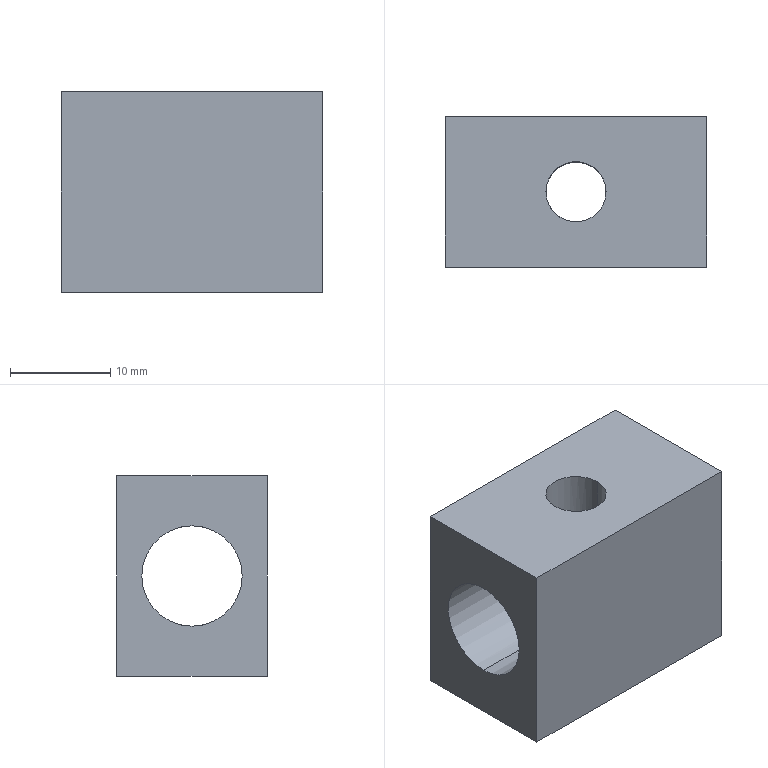Part | SolidWorks | features Extrusion 1, ICE 1 | 1 solid | 12 faces | box 26 x 15 x 20 mm | volume 5462 mm3 | cylinder 6 | plane 6 | commonest cylinder face diameters 6 x4 10 x2
STEP:
#1=CARTESIAN_POINT('',(-13.,0.,15.));
#2=VERTEX_POINT('',#1);
#3=CARTESIAN_POINT('',(-13.,0.,5.));
#4=VERTEX_POINT('',#3);
#5=CARTESIAN_POINT('',(-13.,0.,10.));
#6=DIRECTION('',(1.,0.,0.));
#7=DIRECTION('',(0.,0.,-1.));
#8=AXIS2_PLACEMENT_3D('',#5,#6,#7);
#9=CIRCLE('',#8,5.);
#10=EDGE_CURVE('',#2,#4,#9,.T.);
#11=ORIENTED_EDGE('',*,*,#10,.F.);
#12=CARTESIAN_POINT('',(-3.,0.,15.));
#13=VERTEX_POINT('',#12);
#14=CARTESIAN_POINT('',(-13.,0.,15.));
#15=DIRECTION('',(1.,0.,0.));
#16=VECTOR('',#15,1000.);
#17=LINE('',#14,#16);
#18=EDGE_CURVE('',#2,#13,#17,.T.);
#19=ORIENTED_EDGE('',*,*,#18,.T.);
#20=CARTESIAN_POINT('',(3.,0.,15.));
#21=VERTEX_POINT('',#20);
#22=CARTESIAN_POINT('',(-3.,0.,15.));
#23=CARTESIAN_POINT('',(-3.,-0.2037,15.));
#24=CARTESIAN_POINT('',(-2.979,-0.4031,14.988));
#25=CARTESIAN_POINT('',(-2.9,-0.794,14.94));
#26=CARTESIAN_POINT('',(-2.84,-0.9871,14.905));
#27=CARTESIAN_POINT('',(-2.61,-1.53,14.775));
#28=CARTESIAN_POINT('',(-2.388,-1.856,14.652));
#29=CARTESIAN_POINT('',(-1.982,-2.26,14.463));
#30=CARTESIAN_POINT('',(-1.833,-2.383,14.397));
#31=CARTESIAN_POINT('',(-1.514,-2.597,14.275));
#32=CARTESIAN_POINT('',(-1.346,-2.688,14.217));
#33=CARTESIAN_POINT('',(-0.9876,-2.839,14.117));
#34=CARTESIAN_POINT('',(-0.7957,-2.899,14.074));
#35=CARTESIAN_POINT('',(-0.4054,-2.979,14.016));
#36=CARTESIAN_POINT('',(-0.2042,-3.,14.));
#37=CARTESIAN_POINT('',(0.2022,-3.,14.));
#38=CARTESIAN_POINT('',(0.4015,-2.98,14.015));
#39=CARTESIAN_POINT('',(0.7931,-2.9,14.073));
#40=CARTESIAN_POINT('',(0.9845,-2.841,14.116));
#41=CARTESIAN_POINT('',(1.344,-2.689,14.216));
#42=CARTESIAN_POINT('',(1.516,-2.596,14.275));
#43=CARTESIAN_POINT('',(1.836,-2.381,14.399));
#44=CARTESIAN_POINT('',(1.983,-2.259,14.463));
#45=CARTESIAN_POINT('',(2.255,-1.988,14.59));
#46=CARTESIAN_POINT('',(2.378,-1.839,14.653));
#47=CARTESIAN_POINT('',(2.594,-1.52,14.766));
#48=CARTESIAN_POINT('',(2.686,-1.35,14.818));
#49=CARTESIAN_POINT('',(2.918,-0.8028,14.949));
#50=CARTESIAN_POINT('',(3.,-0.406,15.));
#51=CARTESIAN_POINT('',(3.,0.,15.));
#52=B_SPLINE_CURVE_WITH_KNOTS('',3,(#22,#23,#24,#25,#26,#27,#28,#29,#30,#31,#32,#33,#34,#35,#36,#37,#38,#39,#40,#41,#42,#43,#44,#45,#46,#47,#48,#49,#50,#51),.UNSPECIFIED.,.F.,.F.,(4,2,2,2,2,2,2,2,2,2,2,2,2,2,4),(0.,0.0006015,0.001203,0.002406,0.003008,0.003609,0.004211,0.004812,0.005414,0.006015,0.006617,0.007219,0.00782,0.008422,0.009625),.UNSPECIFIED.);
#53=EDGE_CURVE('',#13,#21,#52,.T.);
#54=ORIENTED_EDGE('',*,*,#53,.T.);
#55=CARTESIAN_POINT('',(13.,0.,15.));
#56=VERTEX_POINT('',#55);
#57=CARTESIAN_POINT('',(-13.,0.,15.));
#58=DIRECTION('',(1.,0.,0.));
#59=VECTOR('',#58,1000.);
#60=LINE('',#57,#59);
#61=EDGE_CURVE('',#21,#56,#60,.T.);
#62=ORIENTED_EDGE('',*,*,#61,.T.);
#63=CARTESIAN_POINT('',(13.,0.,5.));
#64=VERTEX_POINT('',#63);
#65=CARTESIAN_POINT('',(13.,0.,10.));
#66=DIRECTION('',(1.,0.,0.));
#67=DIRECTION('',(0.,0.,-1.));
#68=AXIS2_PLACEMENT_3D('',#65,#66,#67);
#69=CIRCLE('',#68,5.);
#70=EDGE_CURVE('',#56,#64,#69,.T.);
#71=ORIENTED_EDGE('',*,*,#70,.T.);
#72=CARTESIAN_POINT('',(3.,0.,5.));
#73=VERTEX_POINT('',#72);
#74=CARTESIAN_POINT('',(-13.,0.,5.));
#75=DIRECTION('',(1.,0.,0.));
#76=VECTOR('',#75,1000.);
#77=LINE('',#74,#76);
#78=EDGE_CURVE('',#73,#64,#77,.T.);
#79=ORIENTED_EDGE('',*,*,#78,.F.);
#80=CARTESIAN_POINT('',(-3.,0.,5.));
#81=VERTEX_POINT('',#80);
#82=CARTESIAN_POINT('',(3.,0.,5.));
#83=CARTESIAN_POINT('',(3.,-0.2026,5.));
#84=CARTESIAN_POINT('',(2.98,-0.4018,5.012));
#85=CARTESIAN_POINT('',(2.9,-0.7938,5.059));
#86=CARTESIAN_POINT('',(2.84,-0.9867,5.095));
#87=CARTESIAN_POINT('',(2.687,-1.348,5.182));
#88=CARTESIAN_POINT('',(2.593,-1.521,5.234));
#89=CARTESIAN_POINT('',(2.375,-1.843,5.349));
#90=CARTESIAN_POINT('',(2.253,-1.99,5.411));
#91=CARTESIAN_POINT('',(1.982,-2.26,5.537));
#92=CARTESIAN_POINT('',(1.833,-2.383,5.603));
#93=CARTESIAN_POINT('',(1.515,-2.596,5.725));
#94=CARTESIAN_POINT('',(1.347,-2.688,5.783));
#95=CARTESIAN_POINT('',(0.9864,-2.84,5.884));
#96=CARTESIAN_POINT('',(0.7956,-2.899,5.926));
#97=CARTESIAN_POINT('',(0.406,-2.979,5.984));
#98=CARTESIAN_POINT('',(0.2021,-3.,6.));
#99=CARTESIAN_POINT('',(-0.2008,-3.,6.));
#100=CARTESIAN_POINT('',(-0.4,-2.98,5.985));
#101=CARTESIAN_POINT('',(-0.794,-2.9,5.927));
#102=CARTESIAN_POINT('',(-0.9834,-2.841,5.885));
#103=CARTESIAN_POINT('',(-1.344,-2.689,5.784));
#104=CARTESIAN_POINT('',(-1.516,-2.596,5.725));
#105=CARTESIAN_POINT('',(-1.834,-2.382,5.602));
#106=CARTESIAN_POINT('',(-1.982,-2.26,5.538));
#107=CARTESIAN_POINT('',(-2.255,-1.988,5.41));
#108=CARTESIAN_POINT('',(-2.377,-1.84,5.348));
#109=CARTESIAN_POINT('',(-2.592,-1.522,5.234));
#110=CARTESIAN_POINT('',(-2.687,-1.349,5.182));
#111=CARTESIAN_POINT('',(-2.84,-0.9853,5.094));
#112=CARTESIAN_POINT('',(-2.899,-0.797,5.06));
#113=CARTESIAN_POINT('',(-2.979,-0.4074,5.013));
#114=CARTESIAN_POINT('',(-3.,-0.2033,5.));
#115=CARTESIAN_POINT('',(-3.,0.,5.));
#116=B_SPLINE_CURVE_WITH_KNOTS('',3,(#82,#83,#84,#85,#86,#87,#88,#89,#90,#91,#92,#93,#94,#95,#96,#97,#98,#99,#100,#101,#102,#103,#104,#105,#106,#107,#108,#109,#110,#111,#112,#113,#114,#115),.UNSPECIFIED.,.F.,.F.,(4,2,2,2,2,2,2,2,2,2,2,2,2,2,2,2,4),(0.009625,0.01023,0.01083,0.01143,0.01203,0.01263,0.01323,0.01383,0.01443,0.01503,0.01563,0.01623,0.01683,0.01743,0.01803,0.01863,0.01923),.UNSPECIFIED.);
#117=EDGE_CURVE('',#73,#81,#116,.T.);
#118=ORIENTED_EDGE('',*,*,#117,.T.);
#119=CARTESIAN_POINT('',(-13.,0.,5.));
#120=DIRECTION('',(1.,0.,0.));
#121=VECTOR('',#120,1000.);
#122=LINE('',#119,#121);
#123=EDGE_CURVE('',#4,#81,#122,.T.);
#124=ORIENTED_EDGE('',*,*,#123,.F.);
#125=EDGE_LOOP('',(#11,#19,#54,#62,#71,#79,#118,#124));
#126=FACE_OUTER_BOUND('',#125,.T.);
#127=CARTESIAN_POINT('',(-13.,0.,10.));
#128=DIRECTION('',(1.,0.,0.));
#129=DIRECTION('',(0.,0.,-1.));
#130=AXIS2_PLACEMENT_3D('',#127,#128,#129);
#131=CYLINDRICAL_SURFACE('',#130,5.);
#132=ADVANCED_FACE('',(#126),#131,.F.);
#133=ORIENTED_EDGE('',*,*,#117,.F.);
#134=CARTESIAN_POINT('',(3.,0.,0.));
#135=VERTEX_POINT('',#134);
#136=CARTESIAN_POINT('',(3.,0.,20.));
#137=DIRECTION('',(0.,0.,-1.));
#138=VECTOR('',#137,1000.);
#139=LINE('',#136,#138);
#140=EDGE_CURVE('',#73,#135,#139,.T.);
#141=ORIENTED_EDGE('',*,*,#140,.T.);
#142=CARTESIAN_POINT('',(-3.,0.,0.));
#143=VERTEX_POINT('',#142);
#144=CARTESIAN_POINT('',(0.,0.,0.));
#145=DIRECTION('',(0.,0.,1.));
#146=DIRECTION('',(1.,0.,0.));
#147=AXIS2_PLACEMENT_3D('',#144,#145,#146);
#148=CIRCLE('',#147,3.);
#149=EDGE_CURVE('',#143,#135,#148,.T.);
#150=ORIENTED_EDGE('',*,*,#149,.F.);
#151=CARTESIAN_POINT('',(-3.,0.,20.));
#152=DIRECTION('',(0.,0.,-1.));
#153=VECTOR('',#152,1000.);
#154=LINE('',#151,#153);
#155=EDGE_CURVE('',#81,#143,#154,.T.);
#156=ORIENTED_EDGE('',*,*,#155,.F.);
#157=EDGE_LOOP('',(#133,#141,#150,#156));
#158=FACE_OUTER_BOUND('',#157,.T.);
#159=CARTESIAN_POINT('',(0.,0.,20.));
#160=DIRECTION('',(0.,0.,-1.));
#161=DIRECTION('',(-1.,0.,0.));
#162=AXIS2_PLACEMENT_3D('',#159,#160,#161);
#163=CYLINDRICAL_SURFACE('',#162,3.);
#164=ADVANCED_FACE('',(#158),#163,.F.);
#165=CARTESIAN_POINT('',(-3.,0.,20.));
#166=VERTEX_POINT('',#165);
#167=CARTESIAN_POINT('',(3.,0.,20.));
#168=VERTEX_POINT('',#167);
#169=CARTESIAN_POINT('',(0.,0.,20.));
#170=DIRECTION('',(0.,0.,1.));
#171=DIRECTION('',(1.,0.,0.));
#172=AXIS2_PLACEMENT_3D('',#169,#170,#171);
#173=CIRCLE('',#172,3.);
#174=EDGE_CURVE('',#166,#168,#173,.T.);
#175=ORIENTED_EDGE('',*,*,#174,.T.);
#176=CARTESIAN_POINT('',(3.,0.,20.));
#177=DIRECTION('',(0.,0.,-1.));
#178=VECTOR('',#177,1000.);
#179=LINE('',#176,#178);
#180=EDGE_CURVE('',#168,#21,#179,.T.);
#181=ORIENTED_EDGE('',*,*,#180,.T.);
#182=ORIENTED_EDGE('',*,*,#53,.F.);
#183=CARTESIAN_POINT('',(-3.,0.,20.));
#184=DIRECTION('',(0.,0.,-1.));
#185=VECTOR('',#184,1000.);
#186=LINE('',#183,#185);
#187=EDGE_CURVE('',#166,#13,#186,.T.);
#188=ORIENTED_EDGE('',*,*,#187,.F.);
#189=EDGE_LOOP('',(#175,#181,#182,#188));
#190=FACE_OUTER_BOUND('',#189,.T.);
#191=CARTESIAN_POINT('',(0.,0.,20.));
#192=DIRECTION('',(0.,0.,-1.));
#193=DIRECTION('',(-1.,0.,0.));
#194=AXIS2_PLACEMENT_3D('',#191,#192,#193);
#195=CYLINDRICAL_SURFACE('',#194,3.);
#196=ADVANCED_FACE('',(#190),#195,.F.);
#197=ORIENTED_EDGE('',*,*,#180,.F.);
#198=CARTESIAN_POINT('',(0.,0.,20.));
#199=DIRECTION('',(0.,0.,1.));
#200=DIRECTION('',(1.,0.,0.));
#201=AXIS2_PLACEMENT_3D('',#198,#199,#200);
#202=CIRCLE('',#201,3.);
#203=EDGE_CURVE('',#168,#166,#202,.T.);
#204=ORIENTED_EDGE('',*,*,#203,.T.);
#205=ORIENTED_EDGE('',*,*,#187,.T.);
#206=CARTESIAN_POINT('',(3.,0.,15.));
#207=CARTESIAN_POINT('',(3.,0.2026,15.));
#208=CARTESIAN_POINT('',(2.98,0.4018,14.988));
#209=CARTESIAN_POINT('',(2.9,0.7938,14.941));
#210=CARTESIAN_POINT('',(2.84,0.9867,14.905));
#211=CARTESIAN_POINT('',(2.687,1.348,14.818));
#212=CARTESIAN_POINT('',(2.593,1.521,14.766));
#213=CARTESIAN_POINT('',(2.375,1.843,14.651));
#214=CARTESIAN_POINT('',(2.253,1.99,14.589));
#215=CARTESIAN_POINT('',(1.982,2.26,14.463));
#216=CARTESIAN_POINT('',(1.833,2.383,14.397));
#217=CARTESIAN_POINT('',(1.515,2.596,14.275));
#218=CARTESIAN_POINT('',(1.347,2.688,14.217));
#219=CARTESIAN_POINT('',(0.9864,2.84,14.116));
#220=CARTESIAN_POINT('',(0.7956,2.899,14.074));
#221=CARTESIAN_POINT('',(0.406,2.979,14.016));
#222=CARTESIAN_POINT('',(0.2021,3.,14.));
#223=CARTESIAN_POINT('',(-0.2008,3.,14.));
#224=CARTESIAN_POINT('',(-0.4,2.98,14.015));
#225=CARTESIAN_POINT('',(-0.794,2.9,14.073));
#226=CARTESIAN_POINT('',(-0.9834,2.841,14.115));
#227=CARTESIAN_POINT('',(-1.344,2.689,14.216));
#228=CARTESIAN_POINT('',(-1.516,2.596,14.275));
#229=CARTESIAN_POINT('',(-1.834,2.382,14.398));
#230=CARTESIAN_POINT('',(-1.982,2.26,14.462));
#231=CARTESIAN_POINT('',(-2.255,1.988,14.59));
#232=CARTESIAN_POINT('',(-2.377,1.84,14.652));
#233=CARTESIAN_POINT('',(-2.592,1.522,14.766));
#234=CARTESIAN_POINT('',(-2.687,1.349,14.818));
#235=CARTESIAN_POINT('',(-2.84,0.9853,14.906));
#236=CARTESIAN_POINT('',(-2.899,0.797,14.94));
#237=CARTESIAN_POINT('',(-2.979,0.4074,14.987));
#238=CARTESIAN_POINT('',(-3.,0.2033,15.));
#239=CARTESIAN_POINT('',(-3.,0.,15.));
#240=B_SPLINE_CURVE_WITH_KNOTS('',3,(#206,#207,#208,#209,#210,#211,#212,#213,#214,#215,#216,#217,#218,#219,#220,#221,#222,#223,#224,#225,#226,#227,#228,#229,#230,#231,#232,#233,#234,#235,#236,#237,#238,#239),.UNSPECIFIED.,.F.,.F.,(4,2,2,2,2,2,2,2,2,2,2,2,2,2,2,2,4),(0.009625,0.01023,0.01083,0.01143,0.01203,0.01263,0.01323,0.01383,0.01443,0.01503,0.01563,0.01623,0.01683,0.01743,0.01803,0.01863,0.01923),.UNSPECIFIED.);
#241=EDGE_CURVE('',#21,#13,#240,.T.);
#242=ORIENTED_EDGE('',*,*,#241,.F.);
#243=EDGE_LOOP('',(#197,#204,#205,#242));
#244=FACE_OUTER_BOUND('',#243,.T.);
#245=CARTESIAN_POINT('',(0.,0.,20.));
#246=DIRECTION('',(0.,0.,-1.));
#247=DIRECTION('',(-1.,0.,0.));
#248=AXIS2_PLACEMENT_3D('',#245,#246,#247);
#249=CYLINDRICAL_SURFACE('',#248,3.);
#250=ADVANCED_FACE('',(#244),#249,.F.);
#251=CARTESIAN_POINT('',(13.,-7.5,20.));
#252=VERTEX_POINT('',#251);
#253=CARTESIAN_POINT('',(13.,7.5,20.));
#254=VERTEX_POINT('',#253);
#255=CARTESIAN_POINT('',(13.,7.5,20.));
#256=DIRECTION('',(0.,1.,0.));
#257=VECTOR('',#256,1000.);
#258=LINE('',#255,#257);
#259=EDGE_CURVE('',#252,#254,#258,.T.);
#260=ORIENTED_EDGE('',*,*,#259,.T.);
#261=CARTESIAN_POINT('',(-13.,7.5,20.));
#262=VERTEX_POINT('',#261);
#263=CARTESIAN_POINT('',(-13.,7.5,20.));
#264=DIRECTION('',(-1.,0.,0.));
#265=VECTOR('',#264,1000.);
#266=LINE('',#263,#265);
#267=EDGE_CURVE('',#254,#262,#266,.T.);
#268=ORIENTED_EDGE('',*,*,#267,.T.);
#269=CARTESIAN_POINT('',(-13.,-7.5,20.));
#270=VERTEX_POINT('',#269);
#271=CARTESIAN_POINT('',(-13.,7.5,20.));
#272=DIRECTION('',(0.,-1.,0.));
#273=VECTOR('',#272,1000.);
#274=LINE('',#271,#273);
#275=EDGE_CURVE('',#262,#270,#274,.T.);
#276=ORIENTED_EDGE('',*,*,#275,.T.);
#277=CARTESIAN_POINT('',(-13.,-7.5,20.));
#278=DIRECTION('',(1.,0.,0.));
#279=VECTOR('',#278,1000.);
#280=LINE('',#277,#279);
#281=EDGE_CURVE('',#270,#252,#280,.T.);
#282=ORIENTED_EDGE('',*,*,#281,.T.);
#283=EDGE_LOOP('',(#260,#268,#276,#282));
#284=FACE_OUTER_BOUND('',#283,.T.);
#285=ORIENTED_EDGE('',*,*,#174,.F.);
#286=ORIENTED_EDGE('',*,*,#203,.F.);
#287=EDGE_LOOP('',(#285,#286));
#288=FACE_BOUND('',#287,.T.);
#289=CARTESIAN_POINT('',(0.,0.,20.));
#290=DIRECTION('',(0.,0.,1.));
#291=DIRECTION('',(1.,0.,0.));
#292=AXIS2_PLACEMENT_3D('',#289,#290,#291);
#293=PLANE('',#292);
#294=ADVANCED_FACE('',(#284,#288),#293,.T.);
#295=CARTESIAN_POINT('',(13.,-7.5,0.));
#296=VERTEX_POINT('',#295);
#297=CARTESIAN_POINT('',(13.,7.5,0.));
#298=VERTEX_POINT('',#297);
#299=CARTESIAN_POINT('',(13.,7.5,0.));
#300=DIRECTION('',(0.,1.,0.));
#301=VECTOR('',#300,1000.);
#302=LINE('',#299,#301);
#303=EDGE_CURVE('',#296,#298,#302,.T.);
#304=ORIENTED_EDGE('',*,*,#303,.F.);
#305=CARTESIAN_POINT('',(-13.,-7.5,0.));
#306=VERTEX_POINT('',#305);
#307=CARTESIAN_POINT('',(-13.,-7.5,0.));
#308=DIRECTION('',(1.,0.,0.));
#309=VECTOR('',#308,1000.);
#310=LINE('',#307,#309);
#311=EDGE_CURVE('',#306,#296,#310,.T.);
#312=ORIENTED_EDGE('',*,*,#311,.F.);
#313=CARTESIAN_POINT('',(-13.,7.5,0.));
#314=VERTEX_POINT('',#313);
#315=CARTESIAN_POINT('',(-13.,7.5,0.));
#316=DIRECTION('',(0.,-1.,0.));
#317=VECTOR('',#316,1000.);
#318=LINE('',#315,#317);
#319=EDGE_CURVE('',#314,#306,#318,.T.);
#320=ORIENTED_EDGE('',*,*,#319,.F.);
#321=CARTESIAN_POINT('',(-13.,7.5,0.));
#322=DIRECTION('',(-1.,0.,0.));
#323=VECTOR('',#322,1000.);
#324=LINE('',#321,#323);
#325=EDGE_CURVE('',#298,#314,#324,.T.);
#326=ORIENTED_EDGE('',*,*,#325,.F.);
#327=EDGE_LOOP('',(#304,#312,#320,#326));
#328=FACE_OUTER_BOUND('',#327,.T.);
#329=ORIENTED_EDGE('',*,*,#149,.T.);
#330=CARTESIAN_POINT('',(0.,0.,0.));
#331=DIRECTION('',(0.,0.,1.));
#332=DIRECTION('',(1.,0.,0.));
#333=AXIS2_PLACEMENT_3D('',#330,#331,#332);
#334=CIRCLE('',#333,3.);
#335=EDGE_CURVE('',#135,#143,#334,.T.);
#336=ORIENTED_EDGE('',*,*,#335,.T.);
#337=EDGE_LOOP('',(#329,#336));
#338=FACE_BOUND('',#337,.T.);
#339=CARTESIAN_POINT('',(0.,0.,0.));
#340=DIRECTION('',(0.,0.,1.));
#341=DIRECTION('',(1.,0.,0.));
#342=AXIS2_PLACEMENT_3D('',#339,#340,#341);
#343=PLANE('',#342);
#344=ADVANCED_FACE('',(#328,#338),#343,.F.);
#345=CARTESIAN_POINT('',(13.,0.,10.));
#346=DIRECTION('',(1.,0.,0.));
#347=DIRECTION('',(0.,0.,-1.));
#348=AXIS2_PLACEMENT_3D('',#345,#346,#347);
#349=CIRCLE('',#348,5.);
#350=EDGE_CURVE('',#64,#56,#349,.T.);
#351=ORIENTED_EDGE('',*,*,#350,.F.);
#352=ORIENTED_EDGE('',*,*,#70,.F.);
#353=EDGE_LOOP('',(#351,#352));
#354=FACE_BOUND('',#353,.T.);
#355=ORIENTED_EDGE('',*,*,#303,.T.);
#356=CARTESIAN_POINT('',(13.,7.5,20.));
#357=DIRECTION('',(0.,0.,-1.));
#358=VECTOR('',#357,1000.);
#359=LINE('',#356,#358);
#360=EDGE_CURVE('',#254,#298,#359,.T.);
#361=ORIENTED_EDGE('',*,*,#360,.F.);
#362=ORIENTED_EDGE('',*,*,#259,.F.);
#363=CARTESIAN_POINT('',(13.,-7.5,20.));
#364=DIRECTION('',(0.,0.,-1.));
#365=VECTOR('',#364,1000.);
#366=LINE('',#363,#365);
#367=EDGE_CURVE('',#252,#296,#366,.T.);
#368=ORIENTED_EDGE('',*,*,#367,.T.);
#369=EDGE_LOOP('',(#355,#361,#362,#368));
#370=FACE_OUTER_BOUND('',#369,.T.);
#371=CARTESIAN_POINT('',(13.,7.5,20.));
#372=DIRECTION('',(-1.,0.,0.));
#373=DIRECTION('',(0.,0.,1.));
#374=AXIS2_PLACEMENT_3D('',#371,#372,#373);
#375=PLANE('',#374);
#376=ADVANCED_FACE('',(#354,#370),#375,.F.);
#377=ORIENTED_EDGE('',*,*,#325,.T.);
#378=CARTESIAN_POINT('',(-13.,7.5,20.));
#379=DIRECTION('',(0.,0.,-1.));
#380=VECTOR('',#379,1000.);
#381=LINE('',#378,#380);
#382=EDGE_CURVE('',#262,#314,#381,.T.);
#383=ORIENTED_EDGE('',*,*,#382,.F.);
#384=ORIENTED_EDGE('',*,*,#267,.F.);
#385=ORIENTED_EDGE('',*,*,#360,.T.);
#386=EDGE_LOOP('',(#377,#383,#384,#385));
#387=FACE_OUTER_BOUND('',#386,.T.);
#388=CARTESIAN_POINT('',(-13.,7.5,20.));
#389=DIRECTION('',(0.,-1.,0.));
#390=DIRECTION('',(0.,0.,-1.));
#391=AXIS2_PLACEMENT_3D('',#388,#389,#390);
#392=PLANE('',#391);
#393=ADVANCED_FACE('',(#387),#392,.F.);
#394=CARTESIAN_POINT('',(-13.,0.,10.));
#395=DIRECTION('',(1.,0.,0.));
#396=DIRECTION('',(0.,0.,-1.));
#397=AXIS2_PLACEMENT_3D('',#394,#395,#396);
#398=CIRCLE('',#397,5.);
#399=EDGE_CURVE('',#4,#2,#398,.T.);
#400=ORIENTED_EDGE('',*,*,#399,.T.);
#401=ORIENTED_EDGE('',*,*,#10,.T.);
#402=EDGE_LOOP('',(#400,#401));
#403=FACE_BOUND('',#402,.T.);
#404=ORIENTED_EDGE('',*,*,#319,.T.);
#405=CARTESIAN_POINT('',(-13.,-7.5,20.));
#406=DIRECTION('',(0.,0.,-1.));
#407=VECTOR('',#406,1000.);
#408=LINE('',#405,#407);
#409=EDGE_CURVE('',#270,#306,#408,.T.);
#410=ORIENTED_EDGE('',*,*,#409,.F.);
#411=ORIENTED_EDGE('',*,*,#275,.F.);
#412=ORIENTED_EDGE('',*,*,#382,.T.);
#413=EDGE_LOOP('',(#404,#410,#411,#412));
#414=FACE_OUTER_BOUND('',#413,.T.);
#415=CARTESIAN_POINT('',(-13.,7.5,20.));
#416=DIRECTION('',(1.,0.,0.));
#417=DIRECTION('',(0.,1.,0.));
#418=AXIS2_PLACEMENT_3D('',#415,#416,#417);
#419=PLANE('',#418);
#420=ADVANCED_FACE('',(#403,#414),#419,.F.);
#421=ORIENTED_EDGE('',*,*,#311,.T.);
#422=ORIENTED_EDGE('',*,*,#367,.F.);
#423=ORIENTED_EDGE('',*,*,#281,.F.);
#424=ORIENTED_EDGE('',*,*,#409,.T.);
#425=EDGE_LOOP('',(#421,#422,#423,#424));
#426=FACE_OUTER_BOUND('',#425,.T.);
#427=CARTESIAN_POINT('',(-13.,-7.5,20.));
#428=DIRECTION('',(0.,1.,0.));
#429=DIRECTION('',(0.,0.,1.));
#430=AXIS2_PLACEMENT_3D('',#427,#428,#429);
#431=PLANE('',#430);
#432=ADVANCED_FACE('',(#426),#431,.F.);
#433=ORIENTED_EDGE('',*,*,#140,.F.);
#434=CARTESIAN_POINT('',(-3.,0.,5.));
#435=CARTESIAN_POINT('',(-3.,0.2037,5.));
#436=CARTESIAN_POINT('',(-2.979,0.4031,5.012));
#437=CARTESIAN_POINT('',(-2.9,0.794,5.06));
#438=CARTESIAN_POINT('',(-2.84,0.9871,5.095));
#439=CARTESIAN_POINT('',(-2.61,1.53,5.225));
#440=CARTESIAN_POINT('',(-2.388,1.856,5.348));
#441=CARTESIAN_POINT('',(-1.982,2.26,5.537));
#442=CARTESIAN_POINT('',(-1.833,2.383,5.603));
#443=CARTESIAN_POINT('',(-1.514,2.597,5.725));
#444=CARTESIAN_POINT('',(-1.346,2.688,5.783));
#445=CARTESIAN_POINT('',(-0.9876,2.839,5.883));
#446=CARTESIAN_POINT('',(-0.7957,2.899,5.926));
#447=CARTESIAN_POINT('',(-0.4054,2.979,5.984));
#448=CARTESIAN_POINT('',(-0.2042,3.,6.));
#449=CARTESIAN_POINT('',(0.2022,3.,6.));
#450=CARTESIAN_POINT('',(0.4015,2.98,5.985));
#451=CARTESIAN_POINT('',(0.7931,2.9,5.927));
#452=CARTESIAN_POINT('',(0.9845,2.841,5.884));
#453=CARTESIAN_POINT('',(1.344,2.689,5.784));
#454=CARTESIAN_POINT('',(1.516,2.596,5.725));
#455=CARTESIAN_POINT('',(1.836,2.381,5.601));
#456=CARTESIAN_POINT('',(1.983,2.259,5.537));
#457=CARTESIAN_POINT('',(2.255,1.988,5.41));
#458=CARTESIAN_POINT('',(2.378,1.839,5.347));
#459=CARTESIAN_POINT('',(2.594,1.52,5.234));
#460=CARTESIAN_POINT('',(2.686,1.35,5.182));
#461=CARTESIAN_POINT('',(2.918,0.8028,5.051));
#462=CARTESIAN_POINT('',(3.,0.406,5.));
#463=CARTESIAN_POINT('',(3.,0.,5.));
#464=B_SPLINE_CURVE_WITH_KNOTS('',3,(#434,#435,#436,#437,#438,#439,#440,#441,#442,#443,#444,#445,#446,#447,#448,#449,#450,#451,#452,#453,#454,#455,#456,#457,#458,#459,#460,#461,#462,#463),.UNSPECIFIED.,.F.,.F.,(4,2,2,2,2,2,2,2,2,2,2,2,2,2,4),(0.,0.0006015,0.001203,0.002406,0.003008,0.003609,0.004211,0.004812,0.005414,0.006015,0.006617,0.007219,0.00782,0.008422,0.009625),.UNSPECIFIED.);
#465=EDGE_CURVE('',#81,#73,#464,.T.);
#466=ORIENTED_EDGE('',*,*,#465,.F.);
#467=ORIENTED_EDGE('',*,*,#155,.T.);
#468=ORIENTED_EDGE('',*,*,#335,.F.);
#469=EDGE_LOOP('',(#433,#466,#467,#468));
#470=FACE_OUTER_BOUND('',#469,.T.);
#471=CARTESIAN_POINT('',(0.,0.,20.));
#472=DIRECTION('',(0.,0.,-1.));
#473=DIRECTION('',(-1.,0.,0.));
#474=AXIS2_PLACEMENT_3D('',#471,#472,#473);
#475=CYLINDRICAL_SURFACE('',#474,3.);
#476=ADVANCED_FACE('',(#470),#475,.F.);
#477=ORIENTED_EDGE('',*,*,#18,.F.);
#478=ORIENTED_EDGE('',*,*,#399,.F.);
#479=ORIENTED_EDGE('',*,*,#123,.T.);
#480=ORIENTED_EDGE('',*,*,#465,.T.);
#481=ORIENTED_EDGE('',*,*,#78,.T.);
#482=ORIENTED_EDGE('',*,*,#350,.T.);
#483=ORIENTED_EDGE('',*,*,#61,.F.);
#484=ORIENTED_EDGE('',*,*,#241,.T.);
#485=EDGE_LOOP('',(#477,#478,#479,#480,#481,#482,#483,#484));
#486=FACE_OUTER_BOUND('',#485,.T.);
#487=CARTESIAN_POINT('',(-13.,0.,10.));
#488=DIRECTION('',(1.,0.,0.));
#489=DIRECTION('',(0.,0.,-1.));
#490=AXIS2_PLACEMENT_3D('',#487,#488,#489);
#491=CYLINDRICAL_SURFACE('',#490,5.);
#492=ADVANCED_FACE('',(#486),#491,.F.);
#493=CLOSED_SHELL('',(#132,#164,#196,#250,#294,#344,#376,#393,#420,#432,#476,#492));
#494=MANIFOLD_SOLID_BREP('',#493);
#495=CARTESIAN_POINT('',(0.,0.,0.));
#496=DIRECTION('',(0.,0.,1.));
#497=DIRECTION('',(1.,0.,0.));
#498=AXIS2_PLACEMENT_3D('',#495,#496,#497);
#499=(LENGTH_UNIT()NAMED_UNIT(*)SI_UNIT(.MILLI.,.METRE.));
#500=UNCERTAINTY_MEASURE_WITH_UNIT(LENGTH_MEASURE(0.00001),#499,'','');
#501=(NAMED_UNIT(*)PLANE_ANGLE_UNIT()SI_UNIT($,.RADIAN.));
#502=(NAMED_UNIT(*)SI_UNIT($,.STERADIAN.)SOLID_ANGLE_UNIT());
#503=(GEOMETRIC_REPRESENTATION_CONTEXT(3)GLOBAL_UNCERTAINTY_ASSIGNED_CONTEXT((#500))GLOBAL_UNIT_ASSIGNED_CONTEXT((#499,#501,#502))REPRESENTATION_CONTEXT('',''));
#504=ADVANCED_BREP_SHAPE_REPRESENTATION('',(#494,#498),#503);